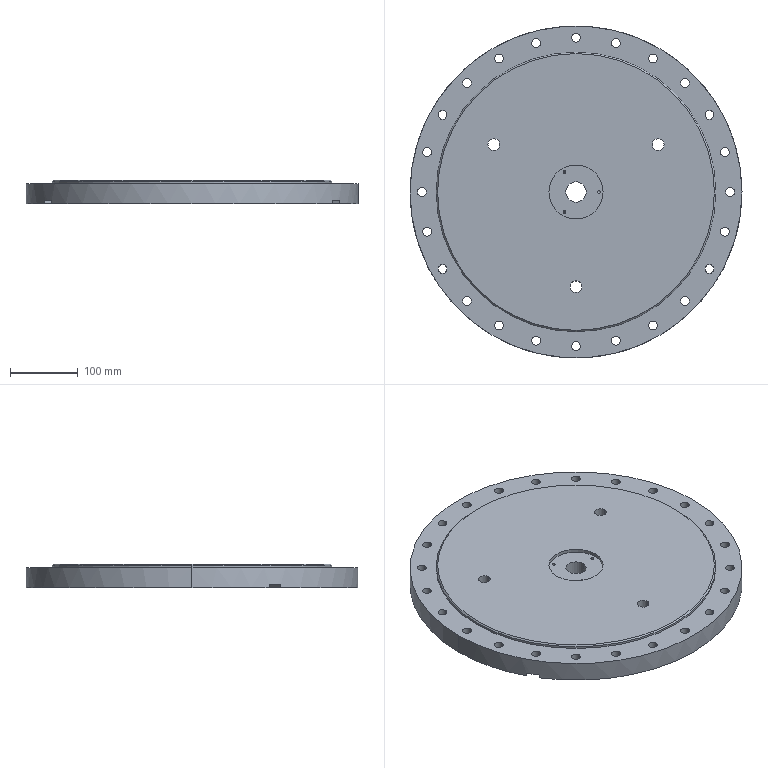Part | SolidWorks | features ICE 5, HoleWzd 4, CirPattern 2, Chamfer 1, Extrusion 1, MirrorPattern 1 | 1 solid | 557 faces | box 490 x 490 x 35 mm | volume 5964420 mm3 | cylinder 308 | cone 200 | plane 49 | commonest cylinder face diameters 5 x168 13 x48 20 x48 4.2 x18 3.2 x12 17.294 x6